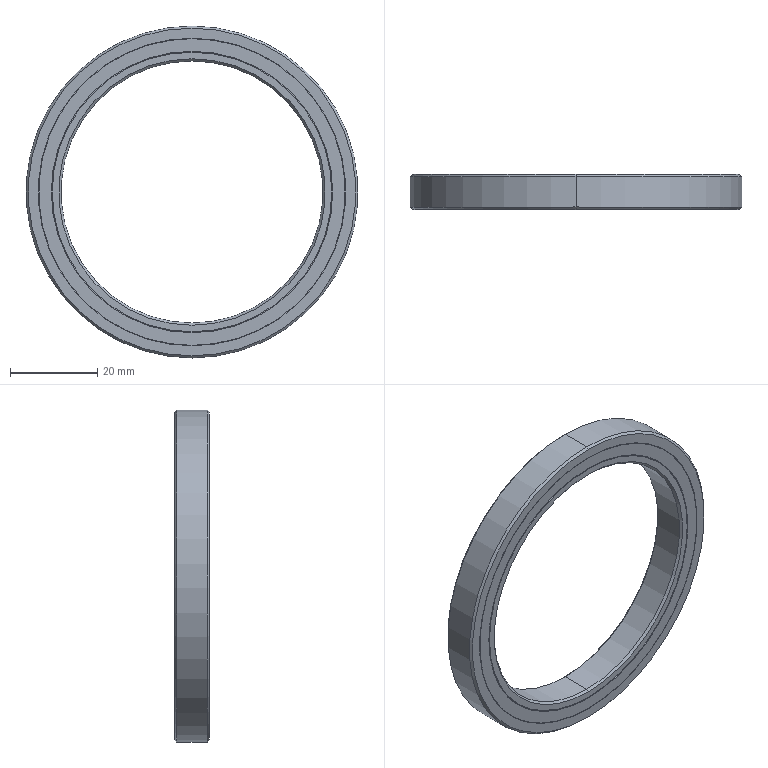Part | SolidWorks | features BaseBody 1 | 1 solid | 38 faces | box 76 x 8 x 76 mm | volume 13540 mm3 | cylinder 20 | plane 10 | cone 8 | commonest cylinder face diameters 64 x4 64.4 x4 70.2 x4 70.4 x4 60 x2 76 x2
STEP:
#1=CARTESIAN_POINT('',(0.,-3.5,38.));
#2=VERTEX_POINT('',#1);
#3=CARTESIAN_POINT('',(0.,-3.5,-38.));
#4=VERTEX_POINT('',#3);
#5=CARTESIAN_POINT('',(0.,-3.5,0.));
#6=DIRECTION('',(0.,1.,0.));
#7=DIRECTION('',(0.,0.,1.));
#8=AXIS2_PLACEMENT_3D('',#5,#6,#7);
#9=CIRCLE('',#8,38.);
#10=EDGE_CURVE('',#2,#4,#9,.T.);
#11=ORIENTED_EDGE('',*,*,#10,.T.);
#12=CARTESIAN_POINT('',(0.,3.5,-38.));
#13=VERTEX_POINT('',#12);
#14=CARTESIAN_POINT('',(0.,60.46,-38.));
#15=DIRECTION('',(0.,1.,0.));
#16=VECTOR('',#15,1000.);
#17=LINE('',#14,#16);
#18=EDGE_CURVE('',#4,#13,#17,.T.);
#19=ORIENTED_EDGE('',*,*,#18,.T.);
#20=CARTESIAN_POINT('',(0.,3.5,38.));
#21=VERTEX_POINT('',#20);
#22=CARTESIAN_POINT('',(0.,3.5,0.));
#23=DIRECTION('',(0.,-1.,0.));
#24=DIRECTION('',(0.,0.,1.));
#25=AXIS2_PLACEMENT_3D('',#22,#23,#24);
#26=CIRCLE('',#25,38.);
#27=EDGE_CURVE('',#13,#21,#26,.T.);
#28=ORIENTED_EDGE('',*,*,#27,.T.);
#29=CARTESIAN_POINT('',(0.,60.46,38.));
#30=DIRECTION('',(0.,1.,0.));
#31=VECTOR('',#30,1000.);
#32=LINE('',#29,#31);
#33=EDGE_CURVE('',#2,#21,#32,.T.);
#34=ORIENTED_EDGE('',*,*,#33,.F.);
#35=EDGE_LOOP('',(#11,#19,#28,#34));
#36=FACE_OUTER_BOUND('',#35,.T.);
#37=CARTESIAN_POINT('',(0.,60.46,0.));
#38=DIRECTION('',(0.,1.,0.));
#39=DIRECTION('',(0.,0.,1.));
#40=AXIS2_PLACEMENT_3D('',#37,#38,#39);
#41=CYLINDRICAL_SURFACE('',#40,38.);
#42=ADVANCED_FACE('',(#36),#41,.T.);
#43=CARTESIAN_POINT('',(0.,4.,-37.5));
#44=VERTEX_POINT('',#43);
#45=CARTESIAN_POINT('',(0.,4.,37.5));
#46=VERTEX_POINT('',#45);
#47=CARTESIAN_POINT('',(0.,4.,0.));
#48=DIRECTION('',(0.,-1.,0.));
#49=DIRECTION('',(0.,0.,-1.));
#50=AXIS2_PLACEMENT_3D('',#47,#48,#49);
#51=CIRCLE('',#50,37.5);
#52=EDGE_CURVE('',#44,#46,#51,.T.);
#53=ORIENTED_EDGE('',*,*,#52,.T.);
#54=CARTESIAN_POINT('',(0.,3.5,38.));
#55=DIRECTION('',(0.,-0.7071,0.7071));
#56=VECTOR('',#55,1000.);
#57=LINE('',#54,#56);
#58=EDGE_CURVE('',#46,#21,#57,.T.);
#59=ORIENTED_EDGE('',*,*,#58,.T.);
#60=ORIENTED_EDGE('',*,*,#27,.F.);
#61=CARTESIAN_POINT('',(0.,3.5,-38.));
#62=DIRECTION('',(0.,-0.7071,-0.7071));
#63=VECTOR('',#62,1000.);
#64=LINE('',#61,#63);
#65=EDGE_CURVE('',#44,#13,#64,.T.);
#66=ORIENTED_EDGE('',*,*,#65,.F.);
#67=EDGE_LOOP('',(#53,#59,#60,#66));
#68=FACE_OUTER_BOUND('',#67,.T.);
#69=CARTESIAN_POINT('',(0.,3.5,0.));
#70=DIRECTION('',(0.,-1.,0.));
#71=DIRECTION('',(0.,0.,-1.));
#72=AXIS2_PLACEMENT_3D('',#69,#70,#71);
#73=CONICAL_SURFACE('',#72,38.,0.7854);
#74=ADVANCED_FACE('',(#68),#73,.T.);
#75=CARTESIAN_POINT('',(0.,-4.,37.5));
#76=VERTEX_POINT('',#75);
#77=CARTESIAN_POINT('',(0.,-4.,-37.5));
#78=VERTEX_POINT('',#77);
#79=CARTESIAN_POINT('',(0.,-4.,0.));
#80=DIRECTION('',(0.,1.,0.));
#81=DIRECTION('',(0.,0.,1.));
#82=AXIS2_PLACEMENT_3D('',#79,#80,#81);
#83=CIRCLE('',#82,37.5);
#84=EDGE_CURVE('',#76,#78,#83,.T.);
#85=ORIENTED_EDGE('',*,*,#84,.T.);
#86=CARTESIAN_POINT('',(0.,-3.5,-38.));
#87=DIRECTION('',(0.,0.7071,-0.7071));
#88=VECTOR('',#87,1000.);
#89=LINE('',#86,#88);
#90=EDGE_CURVE('',#78,#4,#89,.T.);
#91=ORIENTED_EDGE('',*,*,#90,.T.);
#92=ORIENTED_EDGE('',*,*,#10,.F.);
#93=CARTESIAN_POINT('',(0.,-3.5,38.));
#94=DIRECTION('',(0.,0.7071,0.7071));
#95=VECTOR('',#94,1000.);
#96=LINE('',#93,#95);
#97=EDGE_CURVE('',#76,#2,#96,.T.);
#98=ORIENTED_EDGE('',*,*,#97,.F.);
#99=EDGE_LOOP('',(#85,#91,#92,#98));
#100=FACE_OUTER_BOUND('',#99,.T.);
#101=CARTESIAN_POINT('',(0.,-3.5,0.));
#102=DIRECTION('',(0.,1.,0.));
#103=DIRECTION('',(0.,0.,1.));
#104=AXIS2_PLACEMENT_3D('',#101,#102,#103);
#105=CONICAL_SURFACE('',#104,38.,0.7854);
#106=ADVANCED_FACE('',(#100),#105,.T.);
#107=CARTESIAN_POINT('',(0.,3.8,-35.2));
#108=VERTEX_POINT('',#107);
#109=CARTESIAN_POINT('',(0.,3.8,35.2));
#110=VERTEX_POINT('',#109);
#111=CARTESIAN_POINT('',(0.,3.8,0.));
#112=DIRECTION('',(0.,1.,0.));
#113=DIRECTION('',(0.,0.,1.));
#114=AXIS2_PLACEMENT_3D('',#111,#112,#113);
#115=CIRCLE('',#114,35.2);
#116=EDGE_CURVE('',#108,#110,#115,.T.);
#117=ORIENTED_EDGE('',*,*,#116,.F.);
#118=CARTESIAN_POINT('',(0.,4.,-35.2));
#119=VERTEX_POINT('',#118);
#120=CARTESIAN_POINT('',(0.,60.46,-35.2));
#121=DIRECTION('',(0.,1.,0.));
#122=VECTOR('',#121,1000.);
#123=LINE('',#120,#122);
#124=EDGE_CURVE('',#108,#119,#123,.T.);
#125=ORIENTED_EDGE('',*,*,#124,.T.);
#126=CARTESIAN_POINT('',(0.,4.,35.2));
#127=VERTEX_POINT('',#126);
#128=CARTESIAN_POINT('',(0.,4.,0.));
#129=DIRECTION('',(0.,1.,0.));
#130=DIRECTION('',(0.,0.,1.));
#131=AXIS2_PLACEMENT_3D('',#128,#129,#130);
#132=CIRCLE('',#131,35.2);
#133=EDGE_CURVE('',#119,#127,#132,.T.);
#134=ORIENTED_EDGE('',*,*,#133,.T.);
#135=CARTESIAN_POINT('',(0.,60.46,35.2));
#136=DIRECTION('',(0.,1.,0.));
#137=VECTOR('',#136,1000.);
#138=LINE('',#135,#137);
#139=EDGE_CURVE('',#110,#127,#138,.T.);
#140=ORIENTED_EDGE('',*,*,#139,.F.);
#141=EDGE_LOOP('',(#117,#125,#134,#140));
#142=FACE_OUTER_BOUND('',#141,.T.);
#143=CARTESIAN_POINT('',(0.,60.46,0.));
#144=DIRECTION('',(0.,1.,0.));
#145=DIRECTION('',(0.,0.,1.));
#146=AXIS2_PLACEMENT_3D('',#143,#144,#145);
#147=CYLINDRICAL_SURFACE('',#146,35.2);
#148=ADVANCED_FACE('',(#142),#147,.F.);
#149=CARTESIAN_POINT('',(0.,-4.,35.2));
#150=VERTEX_POINT('',#149);
#151=CARTESIAN_POINT('',(0.,-4.,-35.2));
#152=VERTEX_POINT('',#151);
#153=CARTESIAN_POINT('',(0.,-4.,0.));
#154=DIRECTION('',(0.,-1.,0.));
#155=DIRECTION('',(0.,0.,1.));
#156=AXIS2_PLACEMENT_3D('',#153,#154,#155);
#157=CIRCLE('',#156,35.2);
#158=EDGE_CURVE('',#150,#152,#157,.T.);
#159=ORIENTED_EDGE('',*,*,#158,.T.);
#160=CARTESIAN_POINT('',(0.,-3.8,-35.2));
#161=VERTEX_POINT('',#160);
#162=CARTESIAN_POINT('',(0.,60.46,-35.2));
#163=DIRECTION('',(0.,1.,0.));
#164=VECTOR('',#163,1000.);
#165=LINE('',#162,#164);
#166=EDGE_CURVE('',#152,#161,#165,.T.);
#167=ORIENTED_EDGE('',*,*,#166,.T.);
#168=CARTESIAN_POINT('',(0.,-3.8,35.2));
#169=VERTEX_POINT('',#168);
#170=CARTESIAN_POINT('',(0.,-3.8,0.));
#171=DIRECTION('',(0.,-1.,0.));
#172=DIRECTION('',(0.,0.,1.));
#173=AXIS2_PLACEMENT_3D('',#170,#171,#172);
#174=CIRCLE('',#173,35.2);
#175=EDGE_CURVE('',#169,#161,#174,.T.);
#176=ORIENTED_EDGE('',*,*,#175,.F.);
#177=CARTESIAN_POINT('',(0.,60.46,35.2));
#178=DIRECTION('',(0.,1.,0.));
#179=VECTOR('',#178,1000.);
#180=LINE('',#177,#179);
#181=EDGE_CURVE('',#150,#169,#180,.T.);
#182=ORIENTED_EDGE('',*,*,#181,.F.);
#183=EDGE_LOOP('',(#159,#167,#176,#182));
#184=FACE_OUTER_BOUND('',#183,.T.);
#185=CARTESIAN_POINT('',(0.,60.46,0.));
#186=DIRECTION('',(0.,1.,0.));
#187=DIRECTION('',(0.,0.,1.));
#188=AXIS2_PLACEMENT_3D('',#185,#186,#187);
#189=CYLINDRICAL_SURFACE('',#188,35.2);
#190=ADVANCED_FACE('',(#184),#189,.F.);
#191=CARTESIAN_POINT('',(0.,3.8,35.1));
#192=VERTEX_POINT('',#191);
#193=CARTESIAN_POINT('',(0.,3.8,-35.1));
#194=VERTEX_POINT('',#193);
#195=CARTESIAN_POINT('',(0.,3.8,0.));
#196=DIRECTION('',(0.,1.,0.));
#197=DIRECTION('',(0.,0.,1.));
#198=AXIS2_PLACEMENT_3D('',#195,#196,#197);
#199=CIRCLE('',#198,35.1);
#200=EDGE_CURVE('',#192,#194,#199,.T.);
#201=ORIENTED_EDGE('',*,*,#200,.T.);
#202=CARTESIAN_POINT('',(0.,4.,-35.1));
#203=VERTEX_POINT('',#202);
#204=CARTESIAN_POINT('',(0.,60.46,-35.1));
#205=DIRECTION('',(0.,1.,0.));
#206=VECTOR('',#205,1000.);
#207=LINE('',#204,#206);
#208=EDGE_CURVE('',#194,#203,#207,.T.);
#209=ORIENTED_EDGE('',*,*,#208,.T.);
#210=CARTESIAN_POINT('',(0.,4.,35.1));
#211=VERTEX_POINT('',#210);
#212=CARTESIAN_POINT('',(0.,4.,0.));
#213=DIRECTION('',(0.,-1.,0.));
#214=DIRECTION('',(0.,0.,1.));
#215=AXIS2_PLACEMENT_3D('',#212,#213,#214);
#216=CIRCLE('',#215,35.1);
#217=EDGE_CURVE('',#203,#211,#216,.T.);
#218=ORIENTED_EDGE('',*,*,#217,.T.);
#219=CARTESIAN_POINT('',(0.,60.46,35.1));
#220=DIRECTION('',(0.,1.,0.));
#221=VECTOR('',#220,1000.);
#222=LINE('',#219,#221);
#223=EDGE_CURVE('',#192,#211,#222,.T.);
#224=ORIENTED_EDGE('',*,*,#223,.F.);
#225=EDGE_LOOP('',(#201,#209,#218,#224));
#226=FACE_OUTER_BOUND('',#225,.T.);
#227=CARTESIAN_POINT('',(0.,60.46,0.));
#228=DIRECTION('',(0.,1.,0.));
#229=DIRECTION('',(0.,0.,1.));
#230=AXIS2_PLACEMENT_3D('',#227,#228,#229);
#231=CYLINDRICAL_SURFACE('',#230,35.1);
#232=ADVANCED_FACE('',(#226),#231,.T.);
#233=CARTESIAN_POINT('',(0.,-4.,35.1));
#234=VERTEX_POINT('',#233);
#235=CARTESIAN_POINT('',(0.,-4.,-35.1));
#236=VERTEX_POINT('',#235);
#237=CARTESIAN_POINT('',(0.,-4.,0.));
#238=DIRECTION('',(0.,1.,0.));
#239=DIRECTION('',(0.,0.,1.));
#240=AXIS2_PLACEMENT_3D('',#237,#238,#239);
#241=CIRCLE('',#240,35.1);
#242=EDGE_CURVE('',#234,#236,#241,.T.);
#243=ORIENTED_EDGE('',*,*,#242,.T.);
#244=CARTESIAN_POINT('',(0.,-3.8,-35.1));
#245=VERTEX_POINT('',#244);
#246=CARTESIAN_POINT('',(0.,60.46,-35.1));
#247=DIRECTION('',(0.,1.,0.));
#248=VECTOR('',#247,1000.);
#249=LINE('',#246,#248);
#250=EDGE_CURVE('',#236,#245,#249,.T.);
#251=ORIENTED_EDGE('',*,*,#250,.T.);
#252=CARTESIAN_POINT('',(0.,-3.8,35.1));
#253=VERTEX_POINT('',#252);
#254=CARTESIAN_POINT('',(0.,-3.8,0.));
#255=DIRECTION('',(0.,-1.,0.));
#256=DIRECTION('',(0.,0.,1.));
#257=AXIS2_PLACEMENT_3D('',#254,#255,#256);
#258=CIRCLE('',#257,35.1);
#259=EDGE_CURVE('',#245,#253,#258,.T.);
#260=ORIENTED_EDGE('',*,*,#259,.T.);
#261=CARTESIAN_POINT('',(0.,60.46,35.1));
#262=DIRECTION('',(0.,1.,0.));
#263=VECTOR('',#262,1000.);
#264=LINE('',#261,#263);
#265=EDGE_CURVE('',#234,#253,#264,.T.);
#266=ORIENTED_EDGE('',*,*,#265,.F.);
#267=EDGE_LOOP('',(#243,#251,#260,#266));
#268=FACE_OUTER_BOUND('',#267,.T.);
#269=CARTESIAN_POINT('',(0.,60.46,0.));
#270=DIRECTION('',(0.,1.,0.));
#271=DIRECTION('',(0.,0.,1.));
#272=AXIS2_PLACEMENT_3D('',#269,#270,#271);
#273=CYLINDRICAL_SURFACE('',#272,35.1);
#274=ADVANCED_FACE('',(#268),#273,.T.);
#275=CARTESIAN_POINT('',(0.,3.8,-32.2));
#276=VERTEX_POINT('',#275);
#277=CARTESIAN_POINT('',(0.,3.8,32.2));
#278=VERTEX_POINT('',#277);
#279=CARTESIAN_POINT('',(0.,3.8,0.));
#280=DIRECTION('',(0.,1.,0.));
#281=DIRECTION('',(0.,0.,1.));
#282=AXIS2_PLACEMENT_3D('',#279,#280,#281);
#283=CIRCLE('',#282,32.2);
#284=EDGE_CURVE('',#276,#278,#283,.T.);
#285=ORIENTED_EDGE('',*,*,#284,.F.);
#286=CARTESIAN_POINT('',(0.,4.,-32.2));
#287=VERTEX_POINT('',#286);
#288=CARTESIAN_POINT('',(0.,60.46,-32.2));
#289=DIRECTION('',(0.,1.,0.));
#290=VECTOR('',#289,1000.);
#291=LINE('',#288,#290);
#292=EDGE_CURVE('',#276,#287,#291,.T.);
#293=ORIENTED_EDGE('',*,*,#292,.T.);
#294=CARTESIAN_POINT('',(0.,4.,32.2));
#295=VERTEX_POINT('',#294);
#296=CARTESIAN_POINT('',(0.,4.,0.));
#297=DIRECTION('',(0.,1.,0.));
#298=DIRECTION('',(0.,0.,1.));
#299=AXIS2_PLACEMENT_3D('',#296,#297,#298);
#300=CIRCLE('',#299,32.2);
#301=EDGE_CURVE('',#287,#295,#300,.T.);
#302=ORIENTED_EDGE('',*,*,#301,.T.);
#303=CARTESIAN_POINT('',(0.,60.46,32.2));
#304=DIRECTION('',(0.,1.,0.));
#305=VECTOR('',#304,1000.);
#306=LINE('',#303,#305);
#307=EDGE_CURVE('',#278,#295,#306,.T.);
#308=ORIENTED_EDGE('',*,*,#307,.F.);
#309=EDGE_LOOP('',(#285,#293,#302,#308));
#310=FACE_OUTER_BOUND('',#309,.T.);
#311=CARTESIAN_POINT('',(0.,60.46,0.));
#312=DIRECTION('',(0.,1.,0.));
#313=DIRECTION('',(0.,0.,1.));
#314=AXIS2_PLACEMENT_3D('',#311,#312,#313);
#315=CYLINDRICAL_SURFACE('',#314,32.2);
#316=ADVANCED_FACE('',(#310),#315,.F.);
#317=CARTESIAN_POINT('',(0.,-4.,32.2));
#318=VERTEX_POINT('',#317);
#319=CARTESIAN_POINT('',(0.,-4.,-32.2));
#320=VERTEX_POINT('',#319);
#321=CARTESIAN_POINT('',(0.,-4.,0.));
#322=DIRECTION('',(0.,-1.,0.));
#323=DIRECTION('',(0.,0.,1.));
#324=AXIS2_PLACEMENT_3D('',#321,#322,#323);
#325=CIRCLE('',#324,32.2);
#326=EDGE_CURVE('',#318,#320,#325,.T.);
#327=ORIENTED_EDGE('',*,*,#326,.T.);
#328=CARTESIAN_POINT('',(0.,-3.8,-32.2));
#329=VERTEX_POINT('',#328);
#330=CARTESIAN_POINT('',(0.,60.46,-32.2));
#331=DIRECTION('',(0.,1.,0.));
#332=VECTOR('',#331,1000.);
#333=LINE('',#330,#332);
#334=EDGE_CURVE('',#320,#329,#333,.T.);
#335=ORIENTED_EDGE('',*,*,#334,.T.);
#336=CARTESIAN_POINT('',(0.,-3.8,32.2));
#337=VERTEX_POINT('',#336);
#338=CARTESIAN_POINT('',(0.,-3.8,0.));
#339=DIRECTION('',(0.,-1.,0.));
#340=DIRECTION('',(0.,0.,1.));
#341=AXIS2_PLACEMENT_3D('',#338,#339,#340);
#342=CIRCLE('',#341,32.2);
#343=EDGE_CURVE('',#337,#329,#342,.T.);
#344=ORIENTED_EDGE('',*,*,#343,.F.);
#345=CARTESIAN_POINT('',(0.,60.46,32.2));
#346=DIRECTION('',(0.,1.,0.));
#347=VECTOR('',#346,1000.);
#348=LINE('',#345,#347);
#349=EDGE_CURVE('',#318,#337,#348,.T.);
#350=ORIENTED_EDGE('',*,*,#349,.F.);
#351=EDGE_LOOP('',(#327,#335,#344,#350));
#352=FACE_OUTER_BOUND('',#351,.T.);
#353=CARTESIAN_POINT('',(0.,60.46,0.));
#354=DIRECTION('',(0.,1.,0.));
#355=DIRECTION('',(0.,0.,1.));
#356=AXIS2_PLACEMENT_3D('',#353,#354,#355);
#357=CYLINDRICAL_SURFACE('',#356,32.2);
#358=ADVANCED_FACE('',(#352),#357,.F.);
#359=CARTESIAN_POINT('',(0.,3.8,32.));
#360=VERTEX_POINT('',#359);
#361=CARTESIAN_POINT('',(0.,3.8,-32.));
#362=VERTEX_POINT('',#361);
#363=CARTESIAN_POINT('',(0.,3.8,0.));
#364=DIRECTION('',(0.,1.,0.));
#365=DIRECTION('',(0.,0.,1.));
#366=AXIS2_PLACEMENT_3D('',#363,#364,#365);
#367=CIRCLE('',#366,32.);
#368=EDGE_CURVE('',#360,#362,#367,.T.);
#369=ORIENTED_EDGE('',*,*,#368,.T.);
#370=CARTESIAN_POINT('',(0.,4.,-32.));
#371=VERTEX_POINT('',#370);
#372=CARTESIAN_POINT('',(0.,60.46,-32.));
#373=DIRECTION('',(0.,1.,0.));
#374=VECTOR('',#373,1000.);
#375=LINE('',#372,#374);
#376=EDGE_CURVE('',#362,#371,#375,.T.);
#377=ORIENTED_EDGE('',*,*,#376,.T.);
#378=CARTESIAN_POINT('',(0.,4.,32.));
#379=VERTEX_POINT('',#378);
#380=CARTESIAN_POINT('',(0.,4.,0.));
#381=DIRECTION('',(0.,-1.,0.));
#382=DIRECTION('',(0.,0.,1.));
#383=AXIS2_PLACEMENT_3D('',#380,#381,#382);
#384=CIRCLE('',#383,32.);
#385=EDGE_CURVE('',#371,#379,#384,.T.);
#386=ORIENTED_EDGE('',*,*,#385,.T.);
#387=CARTESIAN_POINT('',(0.,60.46,32.));
#388=DIRECTION('',(0.,1.,0.));
#389=VECTOR('',#388,1000.);
#390=LINE('',#387,#389);
#391=EDGE_CURVE('',#360,#379,#390,.T.);
#392=ORIENTED_EDGE('',*,*,#391,.F.);
#393=EDGE_LOOP('',(#369,#377,#386,#392));
#394=FACE_OUTER_BOUND('',#393,.T.);
#395=CARTESIAN_POINT('',(0.,60.46,0.));
#396=DIRECTION('',(0.,1.,0.));
#397=DIRECTION('',(0.,0.,1.));
#398=AXIS2_PLACEMENT_3D('',#395,#396,#397);
#399=CYLINDRICAL_SURFACE('',#398,32.);
#400=ADVANCED_FACE('',(#394),#399,.T.);
#401=CARTESIAN_POINT('',(0.,-4.,32.));
#402=VERTEX_POINT('',#401);
#403=CARTESIAN_POINT('',(0.,-4.,-32.));
#404=VERTEX_POINT('',#403);
#405=CARTESIAN_POINT('',(0.,-4.,0.));
#406=DIRECTION('',(0.,1.,0.));
#407=DIRECTION('',(0.,0.,1.));
#408=AXIS2_PLACEMENT_3D('',#405,#406,#407);
#409=CIRCLE('',#408,32.);
#410=EDGE_CURVE('',#402,#404,#409,.T.);
#411=ORIENTED_EDGE('',*,*,#410,.T.);
#412=CARTESIAN_POINT('',(0.,-3.8,-32.));
#413=VERTEX_POINT('',#412);
#414=CARTESIAN_POINT('',(0.,60.46,-32.));
#415=DIRECTION('',(0.,1.,0.));
#416=VECTOR('',#415,1000.);
#417=LINE('',#414,#416);
#418=EDGE_CURVE('',#404,#413,#417,.T.);
#419=ORIENTED_EDGE('',*,*,#418,.T.);
#420=CARTESIAN_POINT('',(0.,-3.8,32.));
#421=VERTEX_POINT('',#420);
#422=CARTESIAN_POINT('',(0.,-3.8,0.));
#423=DIRECTION('',(0.,-1.,0.));
#424=DIRECTION('',(0.,0.,1.));
#425=AXIS2_PLACEMENT_3D('',#422,#423,#424);
#426=CIRCLE('',#425,32.);
#427=EDGE_CURVE('',#413,#421,#426,.T.);
#428=ORIENTED_EDGE('',*,*,#427,.T.);
#429=CARTESIAN_POINT('',(0.,60.46,32.));
#430=DIRECTION('',(0.,1.,0.));
#431=VECTOR('',#430,1000.);
#432=LINE('',#429,#431);
#433=EDGE_CURVE('',#402,#421,#432,.T.);
#434=ORIENTED_EDGE('',*,*,#433,.F.);
#435=EDGE_LOOP('',(#411,#419,#428,#434));
#436=FACE_OUTER_BOUND('',#435,.T.);
#437=CARTESIAN_POINT('',(0.,60.46,0.));
#438=DIRECTION('',(0.,1.,0.));
#439=DIRECTION('',(0.,0.,1.));
#440=AXIS2_PLACEMENT_3D('',#437,#438,#439);
#441=CYLINDRICAL_SURFACE('',#440,32.);
#442=ADVANCED_FACE('',(#436),#441,.T.);
#443=CARTESIAN_POINT('',(0.,3.5,-30.));
#444=VERTEX_POINT('',#443);
#445=CARTESIAN_POINT('',(0.,3.5,30.));
#446=VERTEX_POINT('',#445);
#447=CARTESIAN_POINT('',(0.,3.5,0.));
#448=DIRECTION('',(0.,1.,0.));
#449=DIRECTION('',(0.,0.,1.));
#450=AXIS2_PLACEMENT_3D('',#447,#448,#449);
#451=CIRCLE('',#450,30.);
#452=EDGE_CURVE('',#444,#446,#451,.T.);
#453=ORIENTED_EDGE('',*,*,#452,.F.);
#454=CARTESIAN_POINT('',(0.,4.,-30.5));
#455=VERTEX_POINT('',#454);
#456=CARTESIAN_POINT('',(0.,4.,-30.5));
#457=DIRECTION('',(0.,0.7071,-0.7071));
#458=VECTOR('',#457,1000.);
#459=LINE('',#456,#458);
#460=EDGE_CURVE('',#444,#455,#459,.T.);
#461=ORIENTED_EDGE('',*,*,#460,.T.);
#462=CARTESIAN_POINT('',(0.,4.,30.5));
#463=VERTEX_POINT('',#462);
#464=CARTESIAN_POINT('',(0.,4.,0.));
#465=DIRECTION('',(0.,1.,0.));
#466=DIRECTION('',(0.,0.,1.));
#467=AXIS2_PLACEMENT_3D('',#464,#465,#466);
#468=CIRCLE('',#467,30.5);
#469=EDGE_CURVE('',#455,#463,#468,.T.);
#470=ORIENTED_EDGE('',*,*,#469,.T.);
#471=CARTESIAN_POINT('',(0.,4.,30.5));
#472=DIRECTION('',(0.,0.7071,0.7071));
#473=VECTOR('',#472,1000.);
#474=LINE('',#471,#473);
#475=EDGE_CURVE('',#446,#463,#474,.T.);
#476=ORIENTED_EDGE('',*,*,#475,.F.);
#477=EDGE_LOOP('',(#453,#461,#470,#476));
#478=FACE_OUTER_BOUND('',#477,.T.);
#479=CARTESIAN_POINT('',(0.,4.,0.));
#480=DIRECTION('',(0.,1.,0.));
#481=DIRECTION('',(0.,0.,1.));
#482=AXIS2_PLACEMENT_3D('',#479,#480,#481);
#483=CONICAL_SURFACE('',#482,30.5,0.7854);
#484=ADVANCED_FACE('',(#478),#483,.F.);
#485=CARTESIAN_POINT('',(0.,-3.5,30.));
#486=VERTEX_POINT('',#485);
#487=CARTESIAN_POINT('',(0.,-3.5,-30.));
#488=VERTEX_POINT('',#487);
#489=CARTESIAN_POINT('',(0.,-3.5,0.));
#490=DIRECTION('',(0.,-1.,0.));
#491=DIRECTION('',(0.,0.,-1.));
#492=AXIS2_PLACEMENT_3D('',#489,#490,#491);
#493=CIRCLE('',#492,30.);
#494=EDGE_CURVE('',#486,#488,#493,.T.);
#495=ORIENTED_EDGE('',*,*,#494,.F.);
#496=CARTESIAN_POINT('',(0.,-4.,30.5));
#497=VERTEX_POINT('',#496);
#498=CARTESIAN_POINT('',(0.,-4.,30.5));
#499=DIRECTION('',(0.,-0.7071,0.7071));
#500=VECTOR('',#499,1000.);
#501=LINE('',#498,#500);
#502=EDGE_CURVE('',#486,#497,#501,.T.);
#503=ORIENTED_EDGE('',*,*,#502,.T.);
#504=CARTESIAN_POINT('',(0.,-4.,-30.5));
#505=VERTEX_POINT('',#504);
#506=CARTESIAN_POINT('',(0.,-4.,0.));
#507=DIRECTION('',(0.,-1.,0.));
#508=DIRECTION('',(0.,0.,-1.));
#509=AXIS2_PLACEMENT_3D('',#506,#507,#508);
#510=CIRCLE('',#509,30.5);
#511=EDGE_CURVE('',#497,#505,#510,.T.);
#512=ORIENTED_EDGE('',*,*,#511,.T.);
#513=CARTESIAN_POINT('',(0.,-4.,-30.5));
#514=DIRECTION('',(0.,-0.7071,-0.7071));
#515=VECTOR('',#514,1000.);
#516=LINE('',#513,#515);
#517=EDGE_CURVE('',#488,#505,#516,.T.);
#518=ORIENTED_EDGE('',*,*,#517,.F.);
#519=EDGE_LOOP('',(#495,#503,#512,#518));
#520=FACE_OUTER_BOUND('',#519,.T.);
#521=CARTESIAN_POINT('',(0.,-4.,0.));
#522=DIRECTION('',(0.,-1.,0.));
#523=DIRECTION('',(0.,0.,-1.));
#524=AXIS2_PLACEMENT_3D('',#521,#522,#523);
#525=CONICAL_SURFACE('',#524,30.5,0.7854);
#526=ADVANCED_FACE('',(#520),#525,.F.);
#527=ORIENTED_EDGE('',*,*,#494,.T.);
#528=CARTESIAN_POINT('',(0.,60.46,-30.));
#529=DIRECTION('',(0.,1.,0.));
#530=VECTOR('',#529,1000.);
#531=LINE('',#528,#530);
#532=EDGE_CURVE('',#488,#444,#531,.T.);
#533=ORIENTED_EDGE('',*,*,#532,.T.);
#534=ORIENTED_EDGE('',*,*,#452,.T.);
#535=CARTESIAN_POINT('',(0.,60.46,30.));
#536=DIRECTION('',(0.,1.,0.));
#537=VECTOR('',#536,1000.);
#538=LINE('',#535,#537);
#539=EDGE_CURVE('',#486,#446,#538,.T.);
#540=ORIENTED_EDGE('',*,*,#539,.F.);
#541=EDGE_LOOP('',(#527,#533,#534,#540));
#542=FACE_OUTER_BOUND('',#541,.T.);
#543=CARTESIAN_POINT('',(0.,60.46,0.));
#544=DIRECTION('',(0.,1.,0.));
#545=DIRECTION('',(0.,0.,1.));
#546=AXIS2_PLACEMENT_3D('',#543,#544,#545);
#547=CYLINDRICAL_SURFACE('',#546,30.);
#548=ADVANCED_FACE('',(#542),#547,.F.);
#549=ORIENTED_EDGE('',*,*,#18,.F.);
#550=CARTESIAN_POINT('',(0.,-3.5,0.));
#551=DIRECTION('',(0.,1.,0.));
#552=DIRECTION('',(0.,0.,1.));
#553=AXIS2_PLACEMENT_3D('',#550,#551,#552);
#554=CIRCLE('',#553,38.);
#555=EDGE_CURVE('',#4,#2,#554,.T.);
#556=ORIENTED_EDGE('',*,*,#555,.T.);
#557=ORIENTED_EDGE('',*,*,#33,.T.);
#558=CARTESIAN_POINT('',(0.,3.5,0.));
#559=DIRECTION('',(0.,-1.,0.));
#560=DIRECTION('',(0.,0.,1.));
#561=AXIS2_PLACEMENT_3D('',#558,#559,#560);
#562=CIRCLE('',#561,38.);
#563=EDGE_CURVE('',#21,#13,#562,.T.);
#564=ORIENTED_EDGE('',*,*,#563,.T.);
#565=EDGE_LOOP('',(#549,#556,#557,#564));
#566=FACE_OUTER_BOUND('',#565,.T.);
#567=CARTESIAN_POINT('',(0.,60.46,0.));
#568=DIRECTION('',(0.,1.,0.));
#569=DIRECTION('',(0.,0.,1.));
#570=AXIS2_PLACEMENT_3D('',#567,#568,#569);
#571=CYLINDRICAL_SURFACE('',#570,38.);
#572=ADVANCED_FACE('',(#566),#571,.T.);
#573=ORIENTED_EDGE('',*,*,#58,.F.);
#574=CARTESIAN_POINT('',(0.,4.,0.));
#575=DIRECTION('',(0.,-1.,0.));
#576=DIRECTION('',(0.,0.,-1.));
#577=AXIS2_PLACEMENT_3D('',#574,#575,#576);
#578=CIRCLE('',#577,37.5);
#579=EDGE_CURVE('',#46,#44,#578,.T.);
#580=ORIENTED_EDGE('',*,*,#579,.T.);
#581=ORIENTED_EDGE('',*,*,#65,.T.);
#582=ORIENTED_EDGE('',*,*,#563,.F.);
#583=EDGE_LOOP('',(#573,#580,#581,#582));
#584=FACE_OUTER_BOUND('',#583,.T.);
#585=CARTESIAN_POINT('',(0.,3.5,0.));
#586=DIRECTION('',(0.,-1.,0.));
#587=DIRECTION('',(0.,0.,-1.));
#588=AXIS2_PLACEMENT_3D('',#585,#586,#587);
#589=CONICAL_SURFACE('',#588,38.,0.7854);
#590=ADVANCED_FACE('',(#584),#589,.T.);
#591=ORIENTED_EDGE('',*,*,#90,.F.);
#592=CARTESIAN_POINT('',(0.,-4.,0.));
#593=DIRECTION('',(0.,1.,0.));
#594=DIRECTION('',(0.,0.,1.));
#595=AXIS2_PLACEMENT_3D('',#592,#593,#594);
#596=CIRCLE('',#595,37.5);
#597=EDGE_CURVE('',#78,#76,#596,.T.);
#598=ORIENTED_EDGE('',*,*,#597,.T.);
#599=ORIENTED_EDGE('',*,*,#97,.T.);
#600=ORIENTED_EDGE('',*,*,#555,.F.);
#601=EDGE_LOOP('',(#591,#598,#599,#600));
#602=FACE_OUTER_BOUND('',#601,.T.);
#603=CARTESIAN_POINT('',(0.,-3.5,0.));
#604=DIRECTION('',(0.,1.,0.));
#605=DIRECTION('',(0.,0.,1.));
#606=AXIS2_PLACEMENT_3D('',#603,#604,#605);
#607=CONICAL_SURFACE('',#606,38.,0.7854);
#608=ADVANCED_FACE('',(#602),#607,.T.);
#609=CARTESIAN_POINT('',(0.,4.,0.));
#610=DIRECTION('',(0.,1.,0.));
#611=DIRECTION('',(0.,0.,1.));
#612=AXIS2_PLACEMENT_3D('',#609,#610,#611);
#613=CIRCLE('',#612,35.2);
#614=EDGE_CURVE('',#127,#119,#613,.T.);
#615=ORIENTED_EDGE('',*,*,#614,.F.);
#616=ORIENTED_EDGE('',*,*,#133,.F.);
#617=EDGE_LOOP('',(#615,#616));
#618=FACE_BOUND('',#617,.T.);
#619=ORIENTED_EDGE('',*,*,#52,.F.);
#620=ORIENTED_EDGE('',*,*,#579,.F.);
#621=EDGE_LOOP('',(#619,#620));
#622=FACE_OUTER_BOUND('',#621,.T.);
#623=CARTESIAN_POINT('',(35.2,4.,0.));
#624=DIRECTION('',(0.,-1.,0.));
#625=DIRECTION('',(0.,0.,-1.));
#626=AXIS2_PLACEMENT_3D('',#623,#624,#625);
#627=PLANE('',#626);
#628=ADVANCED_FACE('',(#618,#622),#627,.F.);
#629=ORIENTED_EDGE('',*,*,#158,.F.);
#630=CARTESIAN_POINT('',(0.,-4.,0.));
#631=DIRECTION('',(0.,-1.,0.));
#632=DIRECTION('',(0.,0.,1.));
#633=AXIS2_PLACEMENT_3D('',#630,#631,#632);
#634=CIRCLE('',#633,35.2);
#635=EDGE_CURVE('',#152,#150,#634,.T.);
#636=ORIENTED_EDGE('',*,*,#635,.F.);
#637=EDGE_LOOP('',(#629,#636));
#638=FACE_BOUND('',#637,.T.);
#639=ORIENTED_EDGE('',*,*,#84,.F.);
#640=ORIENTED_EDGE('',*,*,#597,.F.);
#641=EDGE_LOOP('',(#639,#640));
#642=FACE_OUTER_BOUND('',#641,.T.);
#643=CARTESIAN_POINT('',(35.2,-4.,0.));
#644=DIRECTION('',(0.,1.,0.));
#645=DIRECTION('',(0.,0.,1.));
#646=AXIS2_PLACEMENT_3D('',#643,#644,#645);
#647=PLANE('',#646);
#648=ADVANCED_FACE('',(#638,#642),#647,.F.);
#649=ORIENTED_EDGE('',*,*,#124,.F.);
#650=CARTESIAN_POINT('',(0.,3.8,0.));
#651=DIRECTION('',(0.,1.,0.));
#652=DIRECTION('',(0.,0.,1.));
#653=AXIS2_PLACEMENT_3D('',#650,#651,#652);
#654=CIRCLE('',#653,35.2);
#655=EDGE_CURVE('',#110,#108,#654,.T.);
#656=ORIENTED_EDGE('',*,*,#655,.F.);
#657=ORIENTED_EDGE('',*,*,#139,.T.);
#658=ORIENTED_EDGE('',*,*,#614,.T.);
#659=EDGE_LOOP('',(#649,#656,#657,#658));
#660=FACE_OUTER_BOUND('',#659,.T.);
#661=CARTESIAN_POINT('',(0.,60.46,0.));
#662=DIRECTION('',(0.,1.,0.));
#663=DIRECTION('',(0.,0.,1.));
#664=AXIS2_PLACEMENT_3D('',#661,#662,#663);
#665=CYLINDRICAL_SURFACE('',#664,35.2);
#666=ADVANCED_FACE('',(#660),#665,.F.);
#667=ORIENTED_EDGE('',*,*,#166,.F.);
#668=ORIENTED_EDGE('',*,*,#635,.T.);
#669=ORIENTED_EDGE('',*,*,#181,.T.);
#670=CARTESIAN_POINT('',(0.,-3.8,0.));
#671=DIRECTION('',(0.,-1.,0.));
#672=DIRECTION('',(0.,0.,1.));
#673=AXIS2_PLACEMENT_3D('',#670,#671,#672);
#674=CIRCLE('',#673,35.2);
#675=EDGE_CURVE('',#161,#169,#674,.T.);
#676=ORIENTED_EDGE('',*,*,#675,.F.);
#677=EDGE_LOOP('',(#667,#668,#669,#676));
#678=FACE_OUTER_BOUND('',#677,.T.);
#679=CARTESIAN_POINT('',(0.,60.46,0.));
#680=DIRECTION('',(0.,1.,0.));
#681=DIRECTION('',(0.,0.,1.));
#682=AXIS2_PLACEMENT_3D('',#679,#680,#681);
#683=CYLINDRICAL_SURFACE('',#682,35.2);
#684=ADVANCED_FACE('',(#678),#683,.F.);
#685=ORIENTED_EDGE('',*,*,#655,.T.);
#686=ORIENTED_EDGE('',*,*,#116,.T.);
#687=EDGE_LOOP('',(#685,#686));
#688=FACE_OUTER_BOUND('',#687,.T.);
#689=ORIENTED_EDGE('',*,*,#200,.F.);
#690=CARTESIAN_POINT('',(0.,3.8,0.));
#691=DIRECTION('',(0.,1.,0.));
#692=DIRECTION('',(0.,0.,1.));
#693=AXIS2_PLACEMENT_3D('',#690,#691,#692);
#694=CIRCLE('',#693,35.1);
#695=EDGE_CURVE('',#194,#192,#694,.T.);
#696=ORIENTED_EDGE('',*,*,#695,.F.);
#697=EDGE_LOOP('',(#689,#696));
#698=FACE_BOUND('',#697,.T.);
#699=CARTESIAN_POINT('',(35.1,3.8,0.));
#700=DIRECTION('',(0.,-1.,0.));
#701=DIRECTION('',(0.,0.,-1.));
#702=AXIS2_PLACEMENT_3D('',#699,#700,#701);
#703=PLANE('',#702);
#704=ADVANCED_FACE('',(#688,#698),#703,.F.);
#705=CARTESIAN_POINT('',(0.,-3.8,0.));
#706=DIRECTION('',(0.,-1.,0.));
#707=DIRECTION('',(0.,0.,1.));
#708=AXIS2_PLACEMENT_3D('',#705,#706,#707);
#709=CIRCLE('',#708,35.1);
#710=EDGE_CURVE('',#253,#245,#709,.T.);
#711=ORIENTED_EDGE('',*,*,#710,.F.);
#712=ORIENTED_EDGE('',*,*,#259,.F.);
#713=EDGE_LOOP('',(#711,#712));
#714=FACE_BOUND('',#713,.T.);
#715=ORIENTED_EDGE('',*,*,#175,.T.);
#716=ORIENTED_EDGE('',*,*,#675,.T.);
#717=EDGE_LOOP('',(#715,#716));
#718=FACE_OUTER_BOUND('',#717,.T.);
#719=CARTESIAN_POINT('',(35.1,-3.8,0.));
#720=DIRECTION('',(0.,1.,0.));
#721=DIRECTION('',(0.,0.,1.));
#722=AXIS2_PLACEMENT_3D('',#719,#720,#721);
#723=PLANE('',#722);
#724=ADVANCED_FACE('',(#714,#718),#723,.F.);
#725=ORIENTED_EDGE('',*,*,#208,.F.);
#726=ORIENTED_EDGE('',*,*,#695,.T.);
#727=ORIENTED_EDGE('',*,*,#223,.T.);
#728=CARTESIAN_POINT('',(0.,4.,0.));
#729=DIRECTION('',(0.,-1.,0.));
#730=DIRECTION('',(0.,0.,1.));
#731=AXIS2_PLACEMENT_3D('',#728,#729,#730);
#732=CIRCLE('',#731,35.1);
#733=EDGE_CURVE('',#211,#203,#732,.T.);
#734=ORIENTED_EDGE('',*,*,#733,.T.);
#735=EDGE_LOOP('',(#725,#726,#727,#734));
#736=FACE_OUTER_BOUND('',#735,.T.);
#737=CARTESIAN_POINT('',(0.,60.46,0.));
#738=DIRECTION('',(0.,1.,0.));
#739=DIRECTION('',(0.,0.,1.));
#740=AXIS2_PLACEMENT_3D('',#737,#738,#739);
#741=CYLINDRICAL_SURFACE('',#740,35.1);
#742=ADVANCED_FACE('',(#736),#741,.T.);
#743=ORIENTED_EDGE('',*,*,#250,.F.);
#744=CARTESIAN_POINT('',(0.,-4.,0.));
#745=DIRECTION('',(0.,1.,0.));
#746=DIRECTION('',(0.,0.,1.));
#747=AXIS2_PLACEMENT_3D('',#744,#745,#746);
#748=CIRCLE('',#747,35.1);
#749=EDGE_CURVE('',#236,#234,#748,.T.);
#750=ORIENTED_EDGE('',*,*,#749,.T.);
#751=ORIENTED_EDGE('',*,*,#265,.T.);
#752=ORIENTED_EDGE('',*,*,#710,.T.);
#753=EDGE_LOOP('',(#743,#750,#751,#752));
#754=FACE_OUTER_BOUND('',#753,.T.);
#755=CARTESIAN_POINT('',(0.,60.46,0.));
#756=DIRECTION('',(0.,1.,0.));
#757=DIRECTION('',(0.,0.,1.));
#758=AXIS2_PLACEMENT_3D('',#755,#756,#757);
#759=CYLINDRICAL_SURFACE('',#758,35.1);
#760=ADVANCED_FACE('',(#754),#759,.T.);
#761=ORIENTED_EDGE('',*,*,#733,.F.);
#762=ORIENTED_EDGE('',*,*,#217,.F.);
#763=EDGE_LOOP('',(#761,#762));
#764=FACE_OUTER_BOUND('',#763,.T.);
#765=CARTESIAN_POINT('',(0.,4.,0.));
#766=DIRECTION('',(0.,1.,0.));
#767=DIRECTION('',(0.,0.,1.));
#768=AXIS2_PLACEMENT_3D('',#765,#766,#767);
#769=CIRCLE('',#768,32.2);
#770=EDGE_CURVE('',#295,#287,#769,.T.);
#771=ORIENTED_EDGE('',*,*,#770,.F.);
#772=ORIENTED_EDGE('',*,*,#301,.F.);
#773=EDGE_LOOP('',(#771,#772));
#774=FACE_BOUND('',#773,.T.);
#775=CARTESIAN_POINT('',(32.2,4.,0.));
#776=DIRECTION('',(0.,-1.,0.));
#777=DIRECTION('',(0.,0.,-1.));
#778=AXIS2_PLACEMENT_3D('',#775,#776,#777);
#779=PLANE('',#778);
#780=ADVANCED_FACE('',(#764,#774),#779,.F.);
#781=ORIENTED_EDGE('',*,*,#326,.F.);
#782=CARTESIAN_POINT('',(0.,-4.,0.));
#783=DIRECTION('',(0.,-1.,0.));
#784=DIRECTION('',(0.,0.,1.));
#785=AXIS2_PLACEMENT_3D('',#782,#783,#784);
#786=CIRCLE('',#785,32.2);
#787=EDGE_CURVE('',#320,#318,#786,.T.);
#788=ORIENTED_EDGE('',*,*,#787,.F.);
#789=EDGE_LOOP('',(#781,#788));
#790=FACE_BOUND('',#789,.T.);
#791=ORIENTED_EDGE('',*,*,#242,.F.);
#792=ORIENTED_EDGE('',*,*,#749,.F.);
#793=EDGE_LOOP('',(#791,#792));
#794=FACE_OUTER_BOUND('',#793,.T.);
#795=CARTESIAN_POINT('',(32.2,-4.,0.));
#796=DIRECTION('',(0.,1.,0.));
#797=DIRECTION('',(0.,0.,1.));
#798=AXIS2_PLACEMENT_3D('',#795,#796,#797);
#799=PLANE('',#798);
#800=ADVANCED_FACE('',(#790,#794),#799,.F.);
#801=ORIENTED_EDGE('',*,*,#292,.F.);
#802=CARTESIAN_POINT('',(0.,3.8,0.));
#803=DIRECTION('',(0.,1.,0.));
#804=DIRECTION('',(0.,0.,1.));
#805=AXIS2_PLACEMENT_3D('',#802,#803,#804);
#806=CIRCLE('',#805,32.2);
#807=EDGE_CURVE('',#278,#276,#806,.T.);
#808=ORIENTED_EDGE('',*,*,#807,.F.);
#809=ORIENTED_EDGE('',*,*,#307,.T.);
#810=ORIENTED_EDGE('',*,*,#770,.T.);
#811=EDGE_LOOP('',(#801,#808,#809,#810));
#812=FACE_OUTER_BOUND('',#811,.T.);
#813=CARTESIAN_POINT('',(0.,60.46,0.));
#814=DIRECTION('',(0.,1.,0.));
#815=DIRECTION('',(0.,0.,1.));
#816=AXIS2_PLACEMENT_3D('',#813,#814,#815);
#817=CYLINDRICAL_SURFACE('',#816,32.2);
#818=ADVANCED_FACE('',(#812),#817,.F.);
#819=ORIENTED_EDGE('',*,*,#334,.F.);
#820=ORIENTED_EDGE('',*,*,#787,.T.);
#821=ORIENTED_EDGE('',*,*,#349,.T.);
#822=CARTESIAN_POINT('',(0.,-3.8,0.));
#823=DIRECTION('',(0.,-1.,0.));
#824=DIRECTION('',(0.,0.,1.));
#825=AXIS2_PLACEMENT_3D('',#822,#823,#824);
#826=CIRCLE('',#825,32.2);
#827=EDGE_CURVE('',#329,#337,#826,.T.);
#828=ORIENTED_EDGE('',*,*,#827,.F.);
#829=EDGE_LOOP('',(#819,#820,#821,#828));
#830=FACE_OUTER_BOUND('',#829,.T.);
#831=CARTESIAN_POINT('',(0.,60.46,0.));
#832=DIRECTION('',(0.,1.,0.));
#833=DIRECTION('',(0.,0.,1.));
#834=AXIS2_PLACEMENT_3D('',#831,#832,#833);
#835=CYLINDRICAL_SURFACE('',#834,32.2);
#836=ADVANCED_FACE('',(#830),#835,.F.);
#837=ORIENTED_EDGE('',*,*,#807,.T.);
#838=ORIENTED_EDGE('',*,*,#284,.T.);
#839=EDGE_LOOP('',(#837,#838));
#840=FACE_OUTER_BOUND('',#839,.T.);
#841=ORIENTED_EDGE('',*,*,#368,.F.);
#842=CARTESIAN_POINT('',(0.,3.8,0.));
#843=DIRECTION('',(0.,1.,0.));
#844=DIRECTION('',(0.,0.,1.));
#845=AXIS2_PLACEMENT_3D('',#842,#843,#844);
#846=CIRCLE('',#845,32.);
#847=EDGE_CURVE('',#362,#360,#846,.T.);
#848=ORIENTED_EDGE('',*,*,#847,.F.);
#849=EDGE_LOOP('',(#841,#848));
#850=FACE_BOUND('',#849,.T.);
#851=CARTESIAN_POINT('',(32.,3.8,0.));
#852=DIRECTION('',(0.,-1.,0.));
#853=DIRECTION('',(0.,0.,-1.));
#854=AXIS2_PLACEMENT_3D('',#851,#852,#853);
#855=PLANE('',#854);
#856=ADVANCED_FACE('',(#840,#850),#855,.F.);
#857=CARTESIAN_POINT('',(0.,-3.8,0.));
#858=DIRECTION('',(0.,-1.,0.));
#859=DIRECTION('',(0.,0.,1.));
#860=AXIS2_PLACEMENT_3D('',#857,#858,#859);
#861=CIRCLE('',#860,32.);
#862=EDGE_CURVE('',#421,#413,#861,.T.);
#863=ORIENTED_EDGE('',*,*,#862,.F.);
#864=ORIENTED_EDGE('',*,*,#427,.F.);
#865=EDGE_LOOP('',(#863,#864));
#866=FACE_BOUND('',#865,.T.);
#867=ORIENTED_EDGE('',*,*,#343,.T.);
#868=ORIENTED_EDGE('',*,*,#827,.T.);
#869=EDGE_LOOP('',(#867,#868));
#870=FACE_OUTER_BOUND('',#869,.T.);
#871=CARTESIAN_POINT('',(32.,-3.8,0.));
#872=DIRECTION('',(0.,1.,0.));
#873=DIRECTION('',(0.,0.,1.));
#874=AXIS2_PLACEMENT_3D('',#871,#872,#873);
#875=PLANE('',#874);
#876=ADVANCED_FACE('',(#866,#870),#875,.F.);
#877=ORIENTED_EDGE('',*,*,#376,.F.);
#878=ORIENTED_EDGE('',*,*,#847,.T.);
#879=ORIENTED_EDGE('',*,*,#391,.T.);
#880=CARTESIAN_POINT('',(0.,4.,0.));
#881=DIRECTION('',(0.,-1.,0.));
#882=DIRECTION('',(0.,0.,1.));
#883=AXIS2_PLACEMENT_3D('',#880,#881,#882);
#884=CIRCLE('',#883,32.);
#885=EDGE_CURVE('',#379,#371,#884,.T.);
#886=ORIENTED_EDGE('',*,*,#885,.T.);
#887=EDGE_LOOP('',(#877,#878,#879,#886));
#888=FACE_OUTER_BOUND('',#887,.T.);
#889=CARTESIAN_POINT('',(0.,60.46,0.));
#890=DIRECTION('',(0.,1.,0.));
#891=DIRECTION('',(0.,0.,1.));
#892=AXIS2_PLACEMENT_3D('',#889,#890,#891);
#893=CYLINDRICAL_SURFACE('',#892,32.);
#894=ADVANCED_FACE('',(#888),#893,.T.);
#895=ORIENTED_EDGE('',*,*,#418,.F.);
#896=CARTESIAN_POINT('',(0.,-4.,0.));
#897=DIRECTION('',(0.,1.,0.));
#898=DIRECTION('',(0.,0.,1.));
#899=AXIS2_PLACEMENT_3D('',#896,#897,#898);
#900=CIRCLE('',#899,32.);
#901=EDGE_CURVE('',#404,#402,#900,.T.);
#902=ORIENTED_EDGE('',*,*,#901,.T.);
#903=ORIENTED_EDGE('',*,*,#433,.T.);
#904=ORIENTED_EDGE('',*,*,#862,.T.);
#905=EDGE_LOOP('',(#895,#902,#903,#904));
#906=FACE_OUTER_BOUND('',#905,.T.);
#907=CARTESIAN_POINT('',(0.,60.46,0.));
#908=DIRECTION('',(0.,1.,0.));
#909=DIRECTION('',(0.,0.,1.));
#910=AXIS2_PLACEMENT_3D('',#907,#908,#909);
#911=CYLINDRICAL_SURFACE('',#910,32.);
#912=ADVANCED_FACE('',(#906),#911,.T.);
#913=ORIENTED_EDGE('',*,*,#885,.F.);
#914=ORIENTED_EDGE('',*,*,#385,.F.);
#915=EDGE_LOOP('',(#913,#914));
#916=FACE_OUTER_BOUND('',#915,.T.);
#917=CARTESIAN_POINT('',(0.,4.,0.));
#918=DIRECTION('',(0.,1.,0.));
#919=DIRECTION('',(0.,0.,1.));
#920=AXIS2_PLACEMENT_3D('',#917,#918,#919);
#921=CIRCLE('',#920,30.5);
#922=EDGE_CURVE('',#463,#455,#921,.T.);
#923=ORIENTED_EDGE('',*,*,#922,.F.);
#924=ORIENTED_EDGE('',*,*,#469,.F.);
#925=EDGE_LOOP('',(#923,#924));
#926=FACE_BOUND('',#925,.T.);
#927=CARTESIAN_POINT('',(30.,4.,0.));
#928=DIRECTION('',(0.,-1.,0.));
#929=DIRECTION('',(0.,0.,-1.));
#930=AXIS2_PLACEMENT_3D('',#927,#928,#929);
#931=PLANE('',#930);
#932=ADVANCED_FACE('',(#916,#926),#931,.F.);
#933=ORIENTED_EDGE('',*,*,#410,.F.);
#934=ORIENTED_EDGE('',*,*,#901,.F.);
#935=EDGE_LOOP('',(#933,#934));
#936=FACE_OUTER_BOUND('',#935,.T.);
#937=CARTESIAN_POINT('',(0.,-4.,0.));
#938=DIRECTION('',(0.,-1.,0.));
#939=DIRECTION('',(0.,0.,-1.));
#940=AXIS2_PLACEMENT_3D('',#937,#938,#939);
#941=CIRCLE('',#940,30.5);
#942=EDGE_CURVE('',#505,#497,#941,.T.);
#943=ORIENTED_EDGE('',*,*,#942,.F.);
#944=ORIENTED_EDGE('',*,*,#511,.F.);
#945=EDGE_LOOP('',(#943,#944));
#946=FACE_BOUND('',#945,.T.);
#947=CARTESIAN_POINT('',(30.,-4.,0.));
#948=DIRECTION('',(0.,1.,0.));
#949=DIRECTION('',(0.,0.,1.));
#950=AXIS2_PLACEMENT_3D('',#947,#948,#949);
#951=PLANE('',#950);
#952=ADVANCED_FACE('',(#936,#946),#951,.F.);
#953=ORIENTED_EDGE('',*,*,#460,.F.);
#954=CARTESIAN_POINT('',(0.,3.5,0.));
#955=DIRECTION('',(0.,1.,0.));
#956=DIRECTION('',(0.,0.,1.));
#957=AXIS2_PLACEMENT_3D('',#954,#955,#956);
#958=CIRCLE('',#957,30.);
#959=EDGE_CURVE('',#446,#444,#958,.T.);
#960=ORIENTED_EDGE('',*,*,#959,.F.);
#961=ORIENTED_EDGE('',*,*,#475,.T.);
#962=ORIENTED_EDGE('',*,*,#922,.T.);
#963=EDGE_LOOP('',(#953,#960,#961,#962));
#964=FACE_OUTER_BOUND('',#963,.T.);
#965=CARTESIAN_POINT('',(0.,4.,0.));
#966=DIRECTION('',(0.,1.,0.));
#967=DIRECTION('',(0.,0.,1.));
#968=AXIS2_PLACEMENT_3D('',#965,#966,#967);
#969=CONICAL_SURFACE('',#968,30.5,0.7854);
#970=ADVANCED_FACE('',(#964),#969,.F.);
#971=ORIENTED_EDGE('',*,*,#502,.F.);
#972=CARTESIAN_POINT('',(0.,-3.5,0.));
#973=DIRECTION('',(0.,-1.,0.));
#974=DIRECTION('',(0.,0.,-1.));
#975=AXIS2_PLACEMENT_3D('',#972,#973,#974);
#976=CIRCLE('',#975,30.);
#977=EDGE_CURVE('',#488,#486,#976,.T.);
#978=ORIENTED_EDGE('',*,*,#977,.F.);
#979=ORIENTED_EDGE('',*,*,#517,.T.);
#980=ORIENTED_EDGE('',*,*,#942,.T.);
#981=EDGE_LOOP('',(#971,#978,#979,#980));
#982=FACE_OUTER_BOUND('',#981,.T.);
#983=CARTESIAN_POINT('',(0.,-4.,0.));
#984=DIRECTION('',(0.,-1.,0.));
#985=DIRECTION('',(0.,0.,-1.));
#986=AXIS2_PLACEMENT_3D('',#983,#984,#985);
#987=CONICAL_SURFACE('',#986,30.5,0.7854);
#988=ADVANCED_FACE('',(#982),#987,.F.);
#989=ORIENTED_EDGE('',*,*,#532,.F.);
#990=ORIENTED_EDGE('',*,*,#977,.T.);
#991=ORIENTED_EDGE('',*,*,#539,.T.);
#992=ORIENTED_EDGE('',*,*,#959,.T.);
#993=EDGE_LOOP('',(#989,#990,#991,#992));
#994=FACE_OUTER_BOUND('',#993,.T.);
#995=CARTESIAN_POINT('',(0.,60.46,0.));
#996=DIRECTION('',(0.,1.,0.));
#997=DIRECTION('',(0.,0.,1.));
#998=AXIS2_PLACEMENT_3D('',#995,#996,#997);
#999=CYLINDRICAL_SURFACE('',#998,30.);
#1000=ADVANCED_FACE('',(#994),#999,.F.);
#1001=CLOSED_SHELL('',(#42,#74,#106,#148,#190,#232,#274,#316,#358,#400,#442,#484,#526,#548,#572,#590,#608,#628,#648,#666,#684,#704,#724,#742,#760,#780,#800,#818,#836,#856,#876,#894,#912,#932,#952,#970,#988,#1000));
#1002=MANIFOLD_SOLID_BREP('',#1001);
#1003=CARTESIAN_POINT('',(0.,0.,0.));
#1004=DIRECTION('',(0.,0.,1.));
#1005=DIRECTION('',(1.,0.,0.));
#1006=AXIS2_PLACEMENT_3D('',#1003,#1004,#1005);
#1007=(LENGTH_UNIT()NAMED_UNIT(*)SI_UNIT(.MILLI.,.METRE.));
#1008=UNCERTAINTY_MEASURE_WITH_UNIT(LENGTH_MEASURE(0.00001),#1007,'','');
#1009=(NAMED_UNIT(*)PLANE_ANGLE_UNIT()SI_UNIT($,.RADIAN.));
#1010=(NAMED_UNIT(*)SI_UNIT($,.STERADIAN.)SOLID_ANGLE_UNIT());
#1011=(GEOMETRIC_REPRESENTATION_CONTEXT(3)GLOBAL_UNCERTAINTY_ASSIGNED_CONTEXT((#1008))GLOBAL_UNIT_ASSIGNED_CONTEXT((#1007,#1009,#1010))REPRESENTATION_CONTEXT('',''));
#1012=ADVANCED_BREP_SHAPE_REPRESENTATION('',(#1002,#1006),#1011);